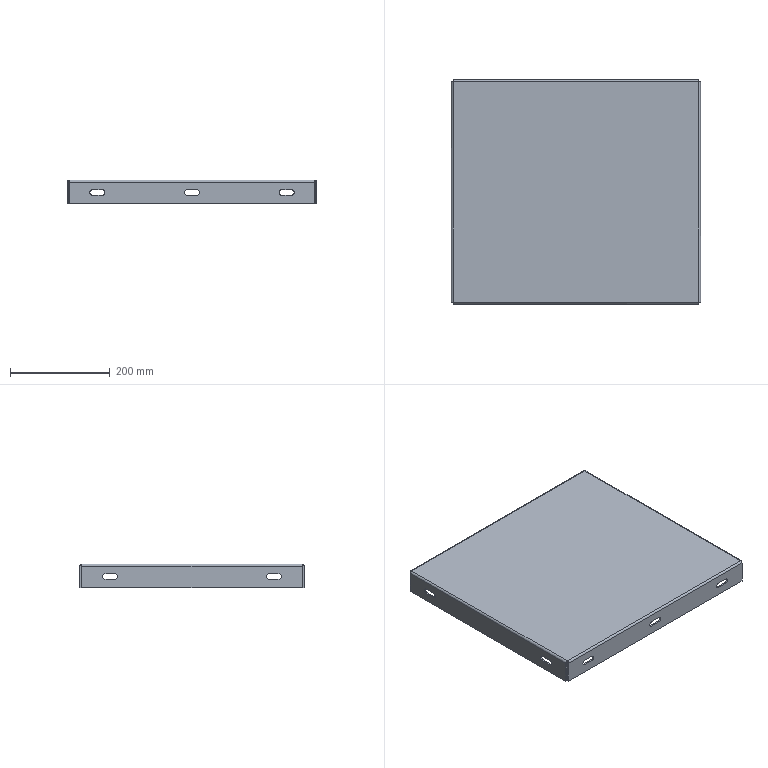Part | NX | features BREP 1 | 1 solid | 78 faces | box 499 x 449 x 48 mm | volume 909026 mm3 | plane 42 | cylinder 28 | spline 8 | commonest cylinder face diameters 10.5 x20 2 x4 8 x4